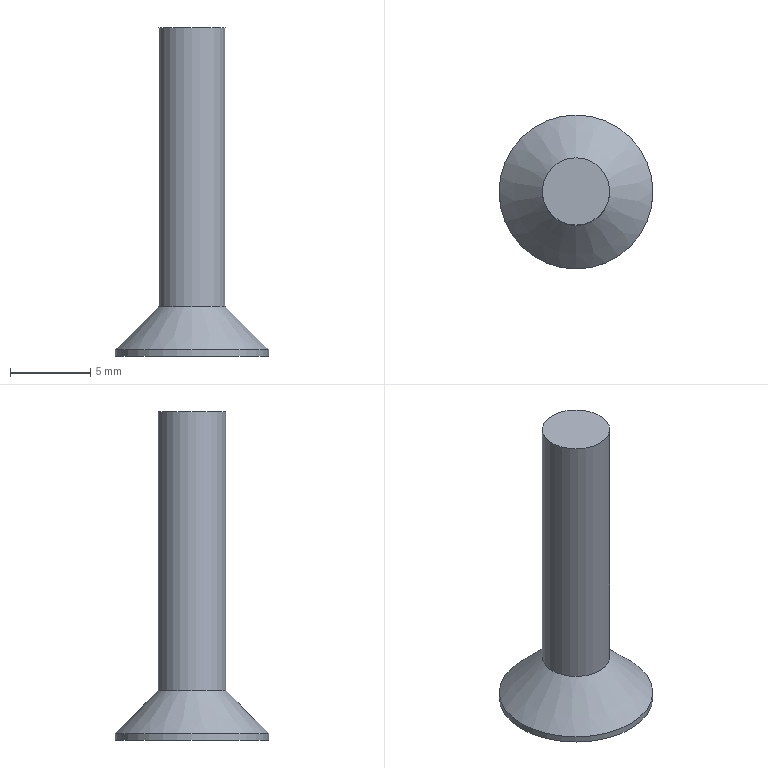Part | NX | features 4 2 | 1 solid | 19 faces | box 9.6 x 9.6 x 20.5 mm | volume 351.436 mm3 | plane 14 | cylinder 3 | cone 2 | commonest cylinder face diameters 3 x1 4.2 x1 9.6 x1
STEP:
#1=CARTESIAN_POINT('',(2130.,344.,22.));
#2=VERTEX_POINT('',#1);
#3=CARTESIAN_POINT('',(2130.,342.5,22.));
#4=DIRECTION('',(0.,0.,1.));
#5=DIRECTION('',(0.,1.,0.));
#6=AXIS2_PLACEMENT_3D('',#3,#4,#5);
#7=CIRCLE('',#6,1.5);
#8=EDGE_CURVE('',#2,#2,#7,.T.);
#9=ORIENTED_EDGE('',*,*,#8,.F.);
#10=EDGE_LOOP('',(#9));
#11=FACE_BOUND('',#10,.T.);
#12=CARTESIAN_POINT('',(2130.,342.5,22.866));
#13=VERTEX_POINT('',#12);
#14=VERTEX_LOOP('',#13);
#15=FACE_BOUND('',#14,.T.);
#16=CARTESIAN_POINT('',(2130.,342.5,22.433));
#17=DIRECTION('',(0.,0.,-1.));
#18=DIRECTION('',(1.,0.,0.));
#19=AXIS2_PLACEMENT_3D('',#16,#17,#18);
#20=CONICAL_SURFACE('',#19,0.75,1.047);
#21=ADVANCED_FACE('',(#11,#15),#20,.F.);
#22=ORIENTED_EDGE('',*,*,#8,.T.);
#23=EDGE_LOOP('',(#22));
#24=FACE_BOUND('',#23,.T.);
#25=CARTESIAN_POINT('',(2131.299,343.25,21.));
#26=VERTEX_POINT('',#25);
#27=CARTESIAN_POINT('',(2130.,344.,21.));
#28=VERTEX_POINT('',#27);
#29=CARTESIAN_POINT('',(2130.,342.5,21.));
#30=DIRECTION('',(0.,0.,1.));
#31=DIRECTION('',(0.,1.,0.));
#32=AXIS2_PLACEMENT_3D('',#29,#30,#31);
#33=CIRCLE('',#32,1.5);
#34=EDGE_CURVE('',#26,#28,#33,.T.);
#35=ORIENTED_EDGE('',*,*,#34,.F.);
#36=CARTESIAN_POINT('',(2131.299,341.75,21.));
#37=VERTEX_POINT('',#36);
#38=CARTESIAN_POINT('',(2130.,342.5,21.));
#39=DIRECTION('',(0.,0.,1.));
#40=DIRECTION('',(0.,1.,0.));
#41=AXIS2_PLACEMENT_3D('',#38,#39,#40);
#42=CIRCLE('',#41,1.5);
#43=EDGE_CURVE('',#37,#26,#42,.T.);
#44=ORIENTED_EDGE('',*,*,#43,.F.);
#45=CARTESIAN_POINT('',(2130.,341.,21.));
#46=VERTEX_POINT('',#45);
#47=CARTESIAN_POINT('',(2130.,342.5,21.));
#48=DIRECTION('',(0.,0.,1.));
#49=DIRECTION('',(0.,1.,0.));
#50=AXIS2_PLACEMENT_3D('',#47,#48,#49);
#51=CIRCLE('',#50,1.5);
#52=EDGE_CURVE('',#46,#37,#51,.T.);
#53=ORIENTED_EDGE('',*,*,#52,.F.);
#54=CARTESIAN_POINT('',(2128.701,341.75,21.));
#55=VERTEX_POINT('',#54);
#56=CARTESIAN_POINT('',(2130.,342.5,21.));
#57=DIRECTION('',(0.,0.,1.));
#58=DIRECTION('',(0.,1.,0.));
#59=AXIS2_PLACEMENT_3D('',#56,#57,#58);
#60=CIRCLE('',#59,1.5);
#61=EDGE_CURVE('',#55,#46,#60,.T.);
#62=ORIENTED_EDGE('',*,*,#61,.F.);
#63=CARTESIAN_POINT('',(2128.701,343.25,21.));
#64=VERTEX_POINT('',#63);
#65=CARTESIAN_POINT('',(2130.,342.5,21.));
#66=DIRECTION('',(0.,0.,1.));
#67=DIRECTION('',(0.,1.,0.));
#68=AXIS2_PLACEMENT_3D('',#65,#66,#67);
#69=CIRCLE('',#68,1.5);
#70=EDGE_CURVE('',#64,#55,#69,.T.);
#71=ORIENTED_EDGE('',*,*,#70,.F.);
#72=CARTESIAN_POINT('',(2130.,342.5,21.));
#73=DIRECTION('',(0.,0.,1.));
#74=DIRECTION('',(0.,1.,0.));
#75=AXIS2_PLACEMENT_3D('',#72,#73,#74);
#76=CIRCLE('',#75,1.5);
#77=EDGE_CURVE('',#28,#64,#76,.T.);
#78=ORIENTED_EDGE('',*,*,#77,.F.);
#79=EDGE_LOOP('',(#35,#44,#53,#62,#71,#78));
#80=FACE_BOUND('',#79,.T.);
#81=CARTESIAN_POINT('',(2130.,342.5,20.5));
#82=DIRECTION('',(0.,0.,1.));
#83=DIRECTION('',(-1.,0.,0.));
#84=AXIS2_PLACEMENT_3D('',#81,#82,#83);
#85=CYLINDRICAL_SURFACE('',#84,1.5);
#86=ADVANCED_FACE('',(#24,#80),#85,.F.);
#87=CARTESIAN_POINT('',(2130.,347.3,19.4));
#88=VERTEX_POINT('',#87);
#89=CARTESIAN_POINT('',(2130.,342.5,19.4));
#90=DIRECTION('',(0.,0.,1.));
#91=DIRECTION('',(0.,1.,0.));
#92=AXIS2_PLACEMENT_3D('',#89,#90,#91);
#93=CIRCLE('',#92,4.8);
#94=EDGE_CURVE('',#88,#88,#93,.T.);
#95=ORIENTED_EDGE('',*,*,#94,.F.);
#96=EDGE_LOOP('',(#95));
#97=FACE_BOUND('',#96,.T.);
#98=CARTESIAN_POINT('',(2130.,347.3,19.));
#99=VERTEX_POINT('',#98);
#100=CARTESIAN_POINT('',(2130.,342.5,19.));
#101=DIRECTION('',(0.,0.,1.));
#102=DIRECTION('',(0.,1.,0.));
#103=AXIS2_PLACEMENT_3D('',#100,#101,#102);
#104=CIRCLE('',#103,4.8);
#105=EDGE_CURVE('',#99,#99,#104,.T.);
#106=ORIENTED_EDGE('',*,*,#105,.T.);
#107=EDGE_LOOP('',(#106));
#108=FACE_BOUND('',#107,.T.);
#109=CARTESIAN_POINT('',(2130.,342.5,19.2));
#110=DIRECTION('',(0.,0.,1.));
#111=DIRECTION('',(-1.,0.,0.));
#112=AXIS2_PLACEMENT_3D('',#109,#110,#111);
#113=CYLINDRICAL_SURFACE('',#112,4.8);
#114=ADVANCED_FACE('',(#97,#108),#113,.T.);
#115=CARTESIAN_POINT('',(2130.,344.6,22.1));
#116=VERTEX_POINT('',#115);
#117=CARTESIAN_POINT('',(2130.,342.5,22.1));
#118=DIRECTION('',(0.,0.,1.));
#119=DIRECTION('',(0.,1.,0.));
#120=AXIS2_PLACEMENT_3D('',#117,#118,#119);
#121=CIRCLE('',#120,2.1);
#122=EDGE_CURVE('',#116,#116,#121,.T.);
#123=ORIENTED_EDGE('',*,*,#122,.F.);
#124=EDGE_LOOP('',(#123));
#125=FACE_BOUND('',#124,.T.);
#126=ORIENTED_EDGE('',*,*,#94,.T.);
#127=EDGE_LOOP('',(#126));
#128=FACE_BOUND('',#127,.T.);
#129=CARTESIAN_POINT('',(2130.,342.5,20.75));
#130=DIRECTION('',(0.,0.,-1.));
#131=DIRECTION('',(1.,0.,0.));
#132=AXIS2_PLACEMENT_3D('',#129,#130,#131);
#133=CONICAL_SURFACE('',#132,3.45,0.7854);
#134=ADVANCED_FACE('',(#125,#128),#133,.T.);
#135=CARTESIAN_POINT('',(2130.,344.6,39.5));
#136=VERTEX_POINT('',#135);
#137=CARTESIAN_POINT('',(2130.,342.5,39.5));
#138=DIRECTION('',(0.,0.,1.));
#139=DIRECTION('',(0.,1.,0.));
#140=AXIS2_PLACEMENT_3D('',#137,#138,#139);
#141=CIRCLE('',#140,2.1);
#142=EDGE_CURVE('',#136,#136,#141,.T.);
#143=ORIENTED_EDGE('',*,*,#142,.F.);
#144=EDGE_LOOP('',(#143));
#145=FACE_BOUND('',#144,.T.);
#146=ORIENTED_EDGE('',*,*,#122,.T.);
#147=EDGE_LOOP('',(#146));
#148=FACE_BOUND('',#147,.T.);
#149=CARTESIAN_POINT('',(2130.,342.5,30.8));
#150=DIRECTION('',(0.,0.,1.));
#151=DIRECTION('',(-1.,0.,0.));
#152=AXIS2_PLACEMENT_3D('',#149,#150,#151);
#153=CYLINDRICAL_SURFACE('',#152,2.1);
#154=ADVANCED_FACE('',(#145,#148),#153,.T.);
#155=CARTESIAN_POINT('',(2130.866,344.,19.));
#156=VERTEX_POINT('',#155);
#157=CARTESIAN_POINT('',(2131.732,342.5,19.));
#158=VERTEX_POINT('',#157);
#159=CARTESIAN_POINT('',(2130.834,344.056,19.));
#160=DIRECTION('',(0.5,-0.866,0.));
#161=VECTOR('',#160,1000.);
#162=LINE('',#159,#161);
#163=EDGE_CURVE('',#156,#158,#162,.T.);
#164=ORIENTED_EDGE('',*,*,#163,.T.);
#165=CARTESIAN_POINT('',(2131.732,342.5,21.));
#166=VERTEX_POINT('',#165);
#167=CARTESIAN_POINT('',(2131.732,342.5,17.));
#168=DIRECTION('',(0.,0.,1.));
#169=VECTOR('',#168,1000.);
#170=LINE('',#167,#169);
#171=EDGE_CURVE('',#158,#166,#170,.T.);
#172=ORIENTED_EDGE('',*,*,#171,.T.);
#173=CARTESIAN_POINT('',(2131.732,342.5,21.));
#174=DIRECTION('',(-0.5,0.866,0.));
#175=VECTOR('',#174,1000.);
#176=LINE('',#173,#175);
#177=EDGE_CURVE('',#166,#26,#176,.T.);
#178=ORIENTED_EDGE('',*,*,#177,.T.);
#179=CARTESIAN_POINT('',(2130.866,344.,21.));
#180=VERTEX_POINT('',#179);
#181=CARTESIAN_POINT('',(2131.732,342.5,21.));
#182=DIRECTION('',(-0.5,0.866,0.));
#183=VECTOR('',#182,1000.);
#184=LINE('',#181,#183);
#185=EDGE_CURVE('',#26,#180,#184,.T.);
#186=ORIENTED_EDGE('',*,*,#185,.T.);
#187=CARTESIAN_POINT('',(2130.866,344.,17.));
#188=DIRECTION('',(0.,0.,1.));
#189=VECTOR('',#188,1000.);
#190=LINE('',#187,#189);
#191=EDGE_CURVE('',#156,#180,#190,.T.);
#192=ORIENTED_EDGE('',*,*,#191,.F.);
#193=EDGE_LOOP('',(#164,#172,#178,#186,#192));
#194=FACE_BOUND('',#193,.T.);
#195=CARTESIAN_POINT('',(2131.732,342.5,17.));
#196=DIRECTION('',(0.866,0.5,0.));
#197=DIRECTION('',(-0.5,0.866,0.));
#198=AXIS2_PLACEMENT_3D('',#195,#196,#197);
#199=PLANE('',#198);
#200=ADVANCED_FACE('',(#194),#199,.F.);
#201=CARTESIAN_POINT('',(2129.134,344.,19.));
#202=VERTEX_POINT('',#201);
#203=CARTESIAN_POINT('',(2130.433,344.,19.));
#204=DIRECTION('',(1.,0.,0.));
#205=VECTOR('',#204,1000.);
#206=LINE('',#203,#205);
#207=EDGE_CURVE('',#202,#156,#206,.T.);
#208=ORIENTED_EDGE('',*,*,#207,.T.);
#209=ORIENTED_EDGE('',*,*,#191,.T.);
#210=CARTESIAN_POINT('',(2130.866,344.,21.));
#211=DIRECTION('',(-1.,0.,0.));
#212=VECTOR('',#211,1000.);
#213=LINE('',#210,#212);
#214=EDGE_CURVE('',#180,#28,#213,.T.);
#215=ORIENTED_EDGE('',*,*,#214,.T.);
#216=CARTESIAN_POINT('',(2129.134,344.,21.));
#217=VERTEX_POINT('',#216);
#218=CARTESIAN_POINT('',(2130.866,344.,21.));
#219=DIRECTION('',(-1.,0.,0.));
#220=VECTOR('',#219,1000.);
#221=LINE('',#218,#220);
#222=EDGE_CURVE('',#28,#217,#221,.T.);
#223=ORIENTED_EDGE('',*,*,#222,.T.);
#224=CARTESIAN_POINT('',(2129.134,344.,17.));
#225=DIRECTION('',(0.,0.,1.));
#226=VECTOR('',#225,1000.);
#227=LINE('',#224,#226);
#228=EDGE_CURVE('',#202,#217,#227,.T.);
#229=ORIENTED_EDGE('',*,*,#228,.F.);
#230=EDGE_LOOP('',(#208,#209,#215,#223,#229));
#231=FACE_BOUND('',#230,.T.);
#232=CARTESIAN_POINT('',(2130.866,344.,17.));
#233=DIRECTION('',(0.,1.,0.));
#234=DIRECTION('',(0.,0.,-1.));
#235=AXIS2_PLACEMENT_3D('',#232,#233,#234);
#236=PLANE('',#235);
#237=ADVANCED_FACE('',(#231),#236,.F.);
#238=CARTESIAN_POINT('',(2130.866,341.,19.));
#239=VERTEX_POINT('',#238);
#240=CARTESIAN_POINT('',(2131.765,342.556,19.));
#241=DIRECTION('',(-0.5,-0.866,0.));
#242=VECTOR('',#241,1000.);
#243=LINE('',#240,#242);
#244=EDGE_CURVE('',#158,#239,#243,.T.);
#245=ORIENTED_EDGE('',*,*,#244,.T.);
#246=CARTESIAN_POINT('',(2130.866,341.,21.));
#247=VERTEX_POINT('',#246);
#248=CARTESIAN_POINT('',(2130.866,341.,17.));
#249=DIRECTION('',(0.,0.,1.));
#250=VECTOR('',#249,1000.);
#251=LINE('',#248,#250);
#252=EDGE_CURVE('',#239,#247,#251,.T.);
#253=ORIENTED_EDGE('',*,*,#252,.T.);
#254=CARTESIAN_POINT('',(2130.866,341.,21.));
#255=DIRECTION('',(0.5,0.866,0.));
#256=VECTOR('',#255,1000.);
#257=LINE('',#254,#256);
#258=EDGE_CURVE('',#247,#37,#257,.T.);
#259=ORIENTED_EDGE('',*,*,#258,.T.);
#260=CARTESIAN_POINT('',(2130.866,341.,21.));
#261=DIRECTION('',(0.5,0.866,0.));
#262=VECTOR('',#261,1000.);
#263=LINE('',#260,#262);
#264=EDGE_CURVE('',#37,#166,#263,.T.);
#265=ORIENTED_EDGE('',*,*,#264,.T.);
#266=ORIENTED_EDGE('',*,*,#171,.F.);
#267=EDGE_LOOP('',(#245,#253,#259,#265,#266));
#268=FACE_BOUND('',#267,.T.);
#269=CARTESIAN_POINT('',(2130.866,341.,17.));
#270=DIRECTION('',(0.866,-0.5,0.));
#271=DIRECTION('',(0.5,0.866,0.));
#272=AXIS2_PLACEMENT_3D('',#269,#270,#271);
#273=PLANE('',#272);
#274=ADVANCED_FACE('',(#268),#273,.F.);
#275=CARTESIAN_POINT('',(2128.268,342.5,19.));
#276=VERTEX_POINT('',#275);
#277=CARTESIAN_POINT('',(2129.599,344.806,19.));
#278=DIRECTION('',(0.5,0.866,0.));
#279=VECTOR('',#278,1000.);
#280=LINE('',#277,#279);
#281=EDGE_CURVE('',#276,#202,#280,.T.);
#282=ORIENTED_EDGE('',*,*,#281,.T.);
#283=ORIENTED_EDGE('',*,*,#228,.T.);
#284=CARTESIAN_POINT('',(2129.134,344.,21.));
#285=DIRECTION('',(-0.5,-0.866,0.));
#286=VECTOR('',#285,1000.);
#287=LINE('',#284,#286);
#288=EDGE_CURVE('',#217,#64,#287,.T.);
#289=ORIENTED_EDGE('',*,*,#288,.T.);
#290=CARTESIAN_POINT('',(2128.268,342.5,21.));
#291=VERTEX_POINT('',#290);
#292=CARTESIAN_POINT('',(2129.134,344.,21.));
#293=DIRECTION('',(-0.5,-0.866,0.));
#294=VECTOR('',#293,1000.);
#295=LINE('',#292,#294);
#296=EDGE_CURVE('',#64,#291,#295,.T.);
#297=ORIENTED_EDGE('',*,*,#296,.T.);
#298=CARTESIAN_POINT('',(2128.268,342.5,17.));
#299=DIRECTION('',(0.,0.,1.));
#300=VECTOR('',#299,1000.);
#301=LINE('',#298,#300);
#302=EDGE_CURVE('',#276,#291,#301,.T.);
#303=ORIENTED_EDGE('',*,*,#302,.F.);
#304=EDGE_LOOP('',(#282,#283,#289,#297,#303));
#305=FACE_BOUND('',#304,.T.);
#306=CARTESIAN_POINT('',(2129.134,344.,17.));
#307=DIRECTION('',(-0.866,0.5,0.));
#308=DIRECTION('',(-0.5,-0.866,0.));
#309=AXIS2_PLACEMENT_3D('',#306,#307,#308);
#310=PLANE('',#309);
#311=ADVANCED_FACE('',(#305),#310,.F.);
#312=ORIENTED_EDGE('',*,*,#61,.T.);
#313=CARTESIAN_POINT('',(2129.134,341.,21.));
#314=VERTEX_POINT('',#313);
#315=CARTESIAN_POINT('',(2129.134,341.,21.));
#316=DIRECTION('',(1.,0.,0.));
#317=VECTOR('',#316,1000.);
#318=LINE('',#315,#317);
#319=EDGE_CURVE('',#314,#46,#318,.T.);
#320=ORIENTED_EDGE('',*,*,#319,.F.);
#321=CARTESIAN_POINT('',(2128.268,342.5,21.));
#322=DIRECTION('',(0.5,-0.866,0.));
#323=VECTOR('',#322,1000.);
#324=LINE('',#321,#323);
#325=EDGE_CURVE('',#55,#314,#324,.T.);
#326=ORIENTED_EDGE('',*,*,#325,.F.);
#327=EDGE_LOOP('',(#312,#320,#326));
#328=FACE_BOUND('',#327,.T.);
#329=CARTESIAN_POINT('',(2130.,342.5,21.));
#330=DIRECTION('',(0.,0.,-1.));
#331=DIRECTION('',(1.,0.,0.));
#332=AXIS2_PLACEMENT_3D('',#329,#330,#331);
#333=PLANE('',#332);
#334=ADVANCED_FACE('',(#328),#333,.T.);
#335=ORIENTED_EDGE('',*,*,#52,.T.);
#336=ORIENTED_EDGE('',*,*,#258,.F.);
#337=CARTESIAN_POINT('',(2129.134,341.,21.));
#338=DIRECTION('',(1.,0.,0.));
#339=VECTOR('',#338,1000.);
#340=LINE('',#337,#339);
#341=EDGE_CURVE('',#46,#247,#340,.T.);
#342=ORIENTED_EDGE('',*,*,#341,.F.);
#343=EDGE_LOOP('',(#335,#336,#342));
#344=FACE_BOUND('',#343,.T.);
#345=CARTESIAN_POINT('',(2130.,342.5,21.));
#346=DIRECTION('',(0.,0.,-1.));
#347=DIRECTION('',(1.,0.,0.));
#348=AXIS2_PLACEMENT_3D('',#345,#346,#347);
#349=PLANE('',#348);
#350=ADVANCED_FACE('',(#344),#349,.T.);
#351=ORIENTED_EDGE('',*,*,#43,.T.);
#352=ORIENTED_EDGE('',*,*,#177,.F.);
#353=ORIENTED_EDGE('',*,*,#264,.F.);
#354=EDGE_LOOP('',(#351,#352,#353));
#355=FACE_BOUND('',#354,.T.);
#356=CARTESIAN_POINT('',(2130.,342.5,21.));
#357=DIRECTION('',(0.,0.,-1.));
#358=DIRECTION('',(1.,0.,0.));
#359=AXIS2_PLACEMENT_3D('',#356,#357,#358);
#360=PLANE('',#359);
#361=ADVANCED_FACE('',(#355),#360,.T.);
#362=ORIENTED_EDGE('',*,*,#34,.T.);
#363=ORIENTED_EDGE('',*,*,#214,.F.);
#364=ORIENTED_EDGE('',*,*,#185,.F.);
#365=EDGE_LOOP('',(#362,#363,#364));
#366=FACE_BOUND('',#365,.T.);
#367=CARTESIAN_POINT('',(2130.,342.5,21.));
#368=DIRECTION('',(0.,0.,-1.));
#369=DIRECTION('',(1.,0.,0.));
#370=AXIS2_PLACEMENT_3D('',#367,#368,#369);
#371=PLANE('',#370);
#372=ADVANCED_FACE('',(#366),#371,.T.);
#373=ORIENTED_EDGE('',*,*,#77,.T.);
#374=ORIENTED_EDGE('',*,*,#288,.F.);
#375=ORIENTED_EDGE('',*,*,#222,.F.);
#376=EDGE_LOOP('',(#373,#374,#375));
#377=FACE_BOUND('',#376,.T.);
#378=CARTESIAN_POINT('',(2130.,342.5,21.));
#379=DIRECTION('',(0.,0.,-1.));
#380=DIRECTION('',(1.,0.,0.));
#381=AXIS2_PLACEMENT_3D('',#378,#379,#380);
#382=PLANE('',#381);
#383=ADVANCED_FACE('',(#377),#382,.T.);
#384=ORIENTED_EDGE('',*,*,#70,.T.);
#385=CARTESIAN_POINT('',(2128.268,342.5,21.));
#386=DIRECTION('',(0.5,-0.866,0.));
#387=VECTOR('',#386,1000.);
#388=LINE('',#385,#387);
#389=EDGE_CURVE('',#291,#55,#388,.T.);
#390=ORIENTED_EDGE('',*,*,#389,.F.);
#391=ORIENTED_EDGE('',*,*,#296,.F.);
#392=EDGE_LOOP('',(#384,#390,#391));
#393=FACE_BOUND('',#392,.T.);
#394=CARTESIAN_POINT('',(2130.,342.5,21.));
#395=DIRECTION('',(0.,0.,-1.));
#396=DIRECTION('',(1.,0.,0.));
#397=AXIS2_PLACEMENT_3D('',#394,#395,#396);
#398=PLANE('',#397);
#399=ADVANCED_FACE('',(#393),#398,.T.);
#400=CARTESIAN_POINT('',(2129.134,341.,19.));
#401=VERTEX_POINT('',#400);
#402=CARTESIAN_POINT('',(2129.567,341.,19.));
#403=DIRECTION('',(-1.,0.,0.));
#404=VECTOR('',#403,1000.);
#405=LINE('',#402,#404);
#406=EDGE_CURVE('',#239,#401,#405,.T.);
#407=ORIENTED_EDGE('',*,*,#406,.T.);
#408=CARTESIAN_POINT('',(2129.134,341.,17.));
#409=DIRECTION('',(0.,0.,1.));
#410=VECTOR('',#409,1000.);
#411=LINE('',#408,#410);
#412=EDGE_CURVE('',#401,#314,#411,.T.);
#413=ORIENTED_EDGE('',*,*,#412,.T.);
#414=ORIENTED_EDGE('',*,*,#319,.T.);
#415=ORIENTED_EDGE('',*,*,#341,.T.);
#416=ORIENTED_EDGE('',*,*,#252,.F.);
#417=EDGE_LOOP('',(#407,#413,#414,#415,#416));
#418=FACE_BOUND('',#417,.T.);
#419=CARTESIAN_POINT('',(2129.134,341.,17.));
#420=DIRECTION('',(0.,-1.,0.));
#421=DIRECTION('',(0.,0.,1.));
#422=AXIS2_PLACEMENT_3D('',#419,#420,#421);
#423=PLANE('',#422);
#424=ADVANCED_FACE('',(#418),#423,.F.);
#425=CARTESIAN_POINT('',(2127.802,343.306,19.));
#426=DIRECTION('',(-0.5,0.866,0.));
#427=VECTOR('',#426,1000.);
#428=LINE('',#425,#427);
#429=EDGE_CURVE('',#401,#276,#428,.T.);
#430=ORIENTED_EDGE('',*,*,#429,.T.);
#431=ORIENTED_EDGE('',*,*,#302,.T.);
#432=ORIENTED_EDGE('',*,*,#389,.T.);
#433=ORIENTED_EDGE('',*,*,#325,.T.);
#434=ORIENTED_EDGE('',*,*,#412,.F.);
#435=EDGE_LOOP('',(#430,#431,#432,#433,#434));
#436=FACE_BOUND('',#435,.T.);
#437=CARTESIAN_POINT('',(2128.268,342.5,17.));
#438=DIRECTION('',(-0.866,-0.5,0.));
#439=DIRECTION('',(0.5,-0.866,0.));
#440=AXIS2_PLACEMENT_3D('',#437,#438,#439);
#441=PLANE('',#440);
#442=ADVANCED_FACE('',(#436),#441,.F.);
#443=ORIENTED_EDGE('',*,*,#142,.T.);
#444=EDGE_LOOP('',(#443));
#445=FACE_BOUND('',#444,.T.);
#446=CARTESIAN_POINT('',(2130.,343.55,39.5));
#447=DIRECTION('',(0.,0.,1.));
#448=DIRECTION('',(-1.,0.,0.));
#449=AXIS2_PLACEMENT_3D('',#446,#447,#448);
#450=PLANE('',#449);
#451=ADVANCED_FACE('',(#445),#450,.T.);
#452=ORIENTED_EDGE('',*,*,#429,.F.);
#453=ORIENTED_EDGE('',*,*,#406,.F.);
#454=ORIENTED_EDGE('',*,*,#244,.F.);
#455=ORIENTED_EDGE('',*,*,#163,.F.);
#456=ORIENTED_EDGE('',*,*,#207,.F.);
#457=ORIENTED_EDGE('',*,*,#281,.F.);
#458=EDGE_LOOP('',(#452,#453,#454,#455,#456,#457));
#459=FACE_BOUND('',#458,.T.);
#460=ORIENTED_EDGE('',*,*,#105,.F.);
#461=EDGE_LOOP('',(#460));
#462=FACE_BOUND('',#461,.T.);
#463=CARTESIAN_POINT('',(2130.,345.65,19.));
#464=DIRECTION('',(0.,0.,-1.));
#465=DIRECTION('',(1.,0.,0.));
#466=AXIS2_PLACEMENT_3D('',#463,#464,#465);
#467=PLANE('',#466);
#468=ADVANCED_FACE('',(#459,#462),#467,.T.);
#469=CLOSED_SHELL('',(#21,#86,#114,#134,#154,#200,#237,#274,#311,#334,#350,#361,#372,#383,#399,#424,#442,#451,#468));
#470=MANIFOLD_SOLID_BREP('',#469);
#471=(LENGTH_UNIT()NAMED_UNIT(*)SI_UNIT(.MILLI.,.METRE.));
#472=UNCERTAINTY_MEASURE_WITH_UNIT(LENGTH_MEASURE(0.00001),#471,'','');
#473=(NAMED_UNIT(*)PLANE_ANGLE_UNIT()SI_UNIT($,.RADIAN.));
#474=(NAMED_UNIT(*)SI_UNIT($,.STERADIAN.)SOLID_ANGLE_UNIT());
#475=(GEOMETRIC_REPRESENTATION_CONTEXT(3)GLOBAL_UNCERTAINTY_ASSIGNED_CONTEXT((#472))GLOBAL_UNIT_ASSIGNED_CONTEXT((#471,#473,#474))REPRESENTATION_CONTEXT('',''));
#476=ADVANCED_BREP_SHAPE_REPRESENTATION('',(#470),#475);